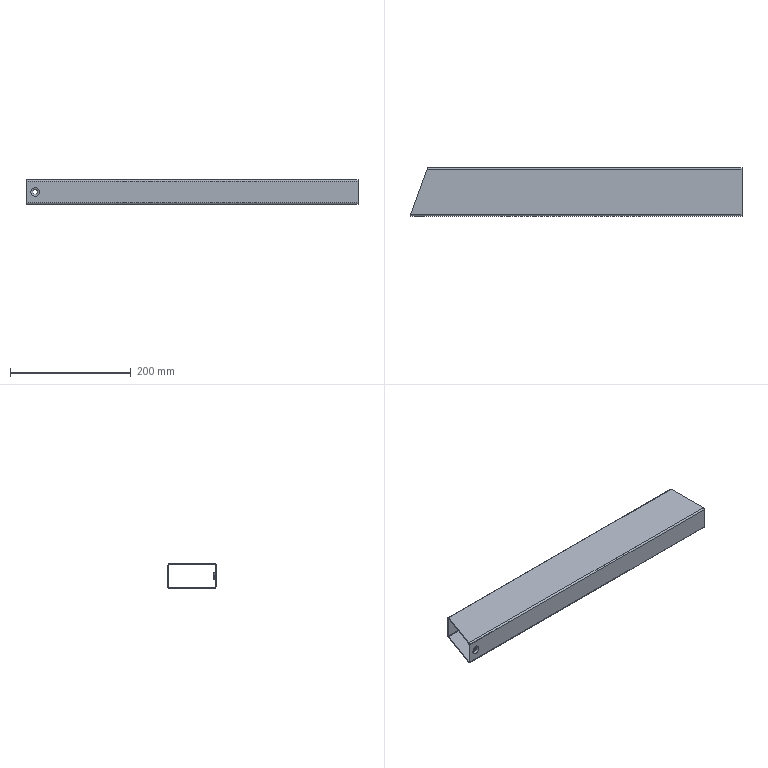Part | STEP file | 5090101 | 1 solid | 23 faces | box 550 x 80 x 40 mm | volume 185626 mm3 | plane 11 | cylinder 10 | torus 2 | commonest cylinder face diameters 2 x4 5 x4 8 x1 11 x1